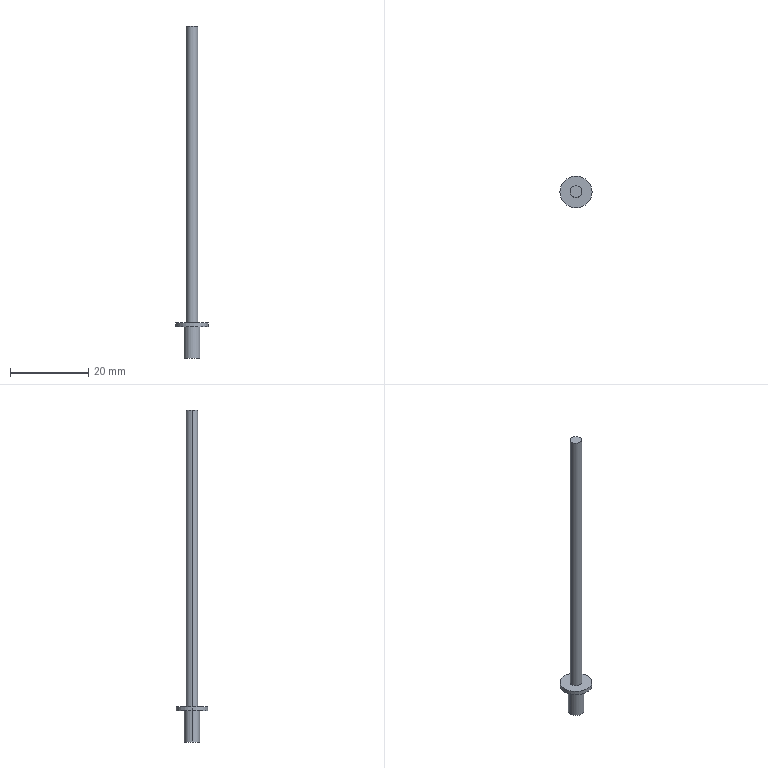Part | Creo | 1 solid | 10 faces | box 8.2 x 8.2 x 85 mm | volume 690.553 mm3 | cylinder 6 | plane 4 | commonest cylinder face diameters 3 x2 4 x2 8.2 x2
STEP:
#1=CARTESIAN_POINT('',(0.,0.,0.));
#2=DIRECTION('',(0.,0.,1.));
#3=DIRECTION('',(1.,0.,0.));
#4=AXIS2_PLACEMENT_3D('',#1,#2,#3);
#5=CARTESIAN_POINT('',(37.6,-82.,-54.09));
#6=VERTEX_POINT('',#5);
#7=CARTESIAN_POINT('',(29.4,-82.,-54.09));
#8=VERTEX_POINT('',#7);
#9=CARTESIAN_POINT('',(33.5,-82.,-54.09));
#10=DIRECTION('',(0.,0.,1.));
#11=DIRECTION('',(1.,0.,0.));
#12=AXIS2_PLACEMENT_3D('',#9,#10,#11);
#13=CIRCLE('',#12,4.1);
#14=EDGE_CURVE('',#6,#8,#13,.T.);
#15=ORIENTED_EDGE('',*,*,#14,.F.);
#16=CARTESIAN_POINT('',(33.5,-82.,-54.09));
#17=DIRECTION('',(0.,0.,1.));
#18=DIRECTION('',(-1.,0.,0.));
#19=AXIS2_PLACEMENT_3D('',#16,#17,#18);
#20=CIRCLE('',#19,4.1);
#21=EDGE_CURVE('',#8,#6,#20,.T.);
#22=ORIENTED_EDGE('',*,*,#21,.F.);
#23=EDGE_LOOP('',(#15,#22));
#24=FACE_OUTER_BOUND('',#23,.F.);
#25=CARTESIAN_POINT('',(35.,-82.,-54.09));
#26=VERTEX_POINT('',#25);
#27=CARTESIAN_POINT('',(32.,-82.,-54.09));
#28=VERTEX_POINT('',#27);
#29=CARTESIAN_POINT('',(33.5,-82.,-54.09));
#30=DIRECTION('',(0.,0.,-1.));
#31=DIRECTION('',(1.,0.,0.));
#32=AXIS2_PLACEMENT_3D('',#29,#30,#31);
#33=CIRCLE('',#32,1.5);
#34=EDGE_CURVE('',#26,#28,#33,.T.);
#35=ORIENTED_EDGE('',*,*,#34,.F.);
#36=CARTESIAN_POINT('',(33.5,-82.,-54.09));
#37=DIRECTION('',(0.,0.,-1.));
#38=DIRECTION('',(-1.,0.,0.));
#39=AXIS2_PLACEMENT_3D('',#36,#37,#38);
#40=CIRCLE('',#39,1.5);
#41=EDGE_CURVE('',#28,#26,#40,.T.);
#42=ORIENTED_EDGE('',*,*,#41,.F.);
#43=EDGE_LOOP('',(#35,#42));
#44=FACE_BOUND('',#43,.F.);
#45=CARTESIAN_POINT('',(33.5,-82.,-54.09));
#46=DIRECTION('',(0.,0.,1.));
#47=DIRECTION('',(1.,0.,0.));
#48=AXIS2_PLACEMENT_3D('',#45,#46,#47);
#49=PLANE('',#48);
#50=ADVANCED_FACE('',(#24,#44),#49,.T.);
#51=ORIENTED_EDGE('',*,*,#14,.T.);
#52=CARTESIAN_POINT('',(29.4,-82.,-55.09));
#53=VERTEX_POINT('',#52);
#54=CARTESIAN_POINT('',(29.4,-82.,-55.09));
#55=DIRECTION('',(0.,0.,1.));
#56=VECTOR('',#55,1.);
#57=LINE('',#54,#56);
#58=EDGE_CURVE('',#53,#8,#57,.T.);
#59=ORIENTED_EDGE('',*,*,#58,.F.);
#60=CARTESIAN_POINT('',(37.6,-82.,-55.09));
#61=VERTEX_POINT('',#60);
#62=CARTESIAN_POINT('',(33.5,-82.,-55.09));
#63=DIRECTION('',(0.,0.,-1.));
#64=DIRECTION('',(-1.,0.,0.));
#65=AXIS2_PLACEMENT_3D('',#62,#63,#64);
#66=CIRCLE('',#65,4.1);
#67=EDGE_CURVE('',#53,#61,#66,.T.);
#68=ORIENTED_EDGE('',*,*,#67,.T.);
#69=CARTESIAN_POINT('',(37.6,-82.,-55.09));
#70=DIRECTION('',(0.,0.,1.));
#71=VECTOR('',#70,1.);
#72=LINE('',#69,#71);
#73=EDGE_CURVE('',#61,#6,#72,.T.);
#74=ORIENTED_EDGE('',*,*,#73,.T.);
#75=EDGE_LOOP('',(#51,#59,#68,#74));
#76=FACE_OUTER_BOUND('',#75,.F.);
#77=CARTESIAN_POINT('',(33.5,-82.,-55.09));
#78=DIRECTION('',(0.,0.,1.));
#79=DIRECTION('',(1.,0.,0.));
#80=AXIS2_PLACEMENT_3D('',#77,#78,#79);
#81=CYLINDRICAL_SURFACE('',#80,4.1);
#82=ADVANCED_FACE('',(#76),#81,.T.);
#83=ORIENTED_EDGE('',*,*,#21,.T.);
#84=ORIENTED_EDGE('',*,*,#73,.F.);
#85=CARTESIAN_POINT('',(33.5,-82.,-55.09));
#86=DIRECTION('',(0.,0.,-1.));
#87=DIRECTION('',(1.,0.,0.));
#88=AXIS2_PLACEMENT_3D('',#85,#86,#87);
#89=CIRCLE('',#88,4.1);
#90=EDGE_CURVE('',#61,#53,#89,.T.);
#91=ORIENTED_EDGE('',*,*,#90,.T.);
#92=ORIENTED_EDGE('',*,*,#58,.T.);
#93=EDGE_LOOP('',(#83,#84,#91,#92));
#94=FACE_OUTER_BOUND('',#93,.F.);
#95=CARTESIAN_POINT('',(33.5,-82.,-55.09));
#96=DIRECTION('',(0.,0.,1.));
#97=DIRECTION('',(1.,0.,0.));
#98=AXIS2_PLACEMENT_3D('',#95,#96,#97);
#99=CYLINDRICAL_SURFACE('',#98,4.1);
#100=ADVANCED_FACE('',(#94),#99,.T.);
#101=ORIENTED_EDGE('',*,*,#90,.F.);
#102=ORIENTED_EDGE('',*,*,#67,.F.);
#103=EDGE_LOOP('',(#101,#102));
#104=FACE_OUTER_BOUND('',#103,.F.);
#105=CARTESIAN_POINT('',(35.5,-82.,-55.09));
#106=VERTEX_POINT('',#105);
#107=CARTESIAN_POINT('',(31.5,-82.,-55.09));
#108=VERTEX_POINT('',#107);
#109=CARTESIAN_POINT('',(33.5,-82.,-55.09));
#110=DIRECTION('',(0.,0.,1.));
#111=DIRECTION('',(1.,0.,0.));
#112=AXIS2_PLACEMENT_3D('',#109,#110,#111);
#113=CIRCLE('',#112,2.);
#114=EDGE_CURVE('',#106,#108,#113,.T.);
#115=ORIENTED_EDGE('',*,*,#114,.F.);
#116=CARTESIAN_POINT('',(33.5,-82.,-55.09));
#117=DIRECTION('',(0.,0.,1.));
#118=DIRECTION('',(-1.,0.,0.));
#119=AXIS2_PLACEMENT_3D('',#116,#117,#118);
#120=CIRCLE('',#119,2.);
#121=EDGE_CURVE('',#108,#106,#120,.T.);
#122=ORIENTED_EDGE('',*,*,#121,.F.);
#123=EDGE_LOOP('',(#115,#122));
#124=FACE_BOUND('',#123,.F.);
#125=CARTESIAN_POINT('',(33.5,-82.,-55.09));
#126=DIRECTION('',(0.,0.,-1.));
#127=DIRECTION('',(-1.,0.,0.));
#128=AXIS2_PLACEMENT_3D('',#125,#126,#127);
#129=PLANE('',#128);
#130=ADVANCED_FACE('',(#104,#124),#129,.T.);
#131=CARTESIAN_POINT('',(31.5,-82.,-63.09));
#132=VERTEX_POINT('',#131);
#133=CARTESIAN_POINT('',(35.5,-82.,-63.09));
#134=VERTEX_POINT('',#133);
#135=CARTESIAN_POINT('',(33.5,-82.,-63.09));
#136=DIRECTION('',(0.,0.,-1.));
#137=DIRECTION('',(-1.,0.,0.));
#138=AXIS2_PLACEMENT_3D('',#135,#136,#137);
#139=CIRCLE('',#138,2.);
#140=EDGE_CURVE('',#132,#134,#139,.T.);
#141=ORIENTED_EDGE('',*,*,#140,.T.);
#142=CARTESIAN_POINT('',(35.5,-82.,-63.09));
#143=DIRECTION('',(0.,0.,1.));
#144=VECTOR('',#143,8.);
#145=LINE('',#142,#144);
#146=EDGE_CURVE('',#134,#106,#145,.T.);
#147=ORIENTED_EDGE('',*,*,#146,.T.);
#148=ORIENTED_EDGE('',*,*,#114,.T.);
#149=CARTESIAN_POINT('',(31.5,-82.,-63.09));
#150=DIRECTION('',(0.,0.,1.));
#151=VECTOR('',#150,8.);
#152=LINE('',#149,#151);
#153=EDGE_CURVE('',#132,#108,#152,.T.);
#154=ORIENTED_EDGE('',*,*,#153,.F.);
#155=EDGE_LOOP('',(#141,#147,#148,#154));
#156=FACE_OUTER_BOUND('',#155,.F.);
#157=CARTESIAN_POINT('',(33.5,-82.,-90.09));
#158=DIRECTION('',(0.,0.,1.));
#159=DIRECTION('',(1.,0.,0.));
#160=AXIS2_PLACEMENT_3D('',#157,#158,#159);
#161=CYLINDRICAL_SURFACE('',#160,2.);
#162=ADVANCED_FACE('',(#156),#161,.T.);
#163=CARTESIAN_POINT('',(33.5,-82.,-63.09));
#164=DIRECTION('',(0.,0.,-1.));
#165=DIRECTION('',(1.,0.,0.));
#166=AXIS2_PLACEMENT_3D('',#163,#164,#165);
#167=CIRCLE('',#166,2.);
#168=EDGE_CURVE('',#134,#132,#167,.T.);
#169=ORIENTED_EDGE('',*,*,#168,.F.);
#170=ORIENTED_EDGE('',*,*,#140,.F.);
#171=EDGE_LOOP('',(#169,#170));
#172=FACE_OUTER_BOUND('',#171,.F.);
#173=CARTESIAN_POINT('',(-38.5,-81.,-63.09));
#174=DIRECTION('',(0.,0.,1.));
#175=DIRECTION('',(1.,0.,0.));
#176=AXIS2_PLACEMENT_3D('',#173,#174,#175);
#177=PLANE('',#176);
#178=ADVANCED_FACE('',(#172),#177,.F.);
#179=ORIENTED_EDGE('',*,*,#168,.T.);
#180=ORIENTED_EDGE('',*,*,#153,.T.);
#181=ORIENTED_EDGE('',*,*,#121,.T.);
#182=ORIENTED_EDGE('',*,*,#146,.F.);
#183=EDGE_LOOP('',(#179,#180,#181,#182));
#184=FACE_OUTER_BOUND('',#183,.F.);
#185=CARTESIAN_POINT('',(33.5,-82.,-90.09));
#186=DIRECTION('',(0.,0.,1.));
#187=DIRECTION('',(1.,0.,0.));
#188=AXIS2_PLACEMENT_3D('',#185,#186,#187);
#189=CYLINDRICAL_SURFACE('',#188,2.);
#190=ADVANCED_FACE('',(#184),#189,.T.);
#191=ORIENTED_EDGE('',*,*,#34,.T.);
#192=CARTESIAN_POINT('',(32.,-82.,21.91));
#193=VERTEX_POINT('',#192);
#194=CARTESIAN_POINT('',(32.,-82.,21.91));
#195=DIRECTION('',(0.,0.,-1.));
#196=VECTOR('',#195,76.);
#197=LINE('',#194,#196);
#198=EDGE_CURVE('',#193,#28,#197,.T.);
#199=ORIENTED_EDGE('',*,*,#198,.F.);
#200=CARTESIAN_POINT('',(35.,-82.,21.91));
#201=VERTEX_POINT('',#200);
#202=CARTESIAN_POINT('',(33.5,-82.,21.91));
#203=DIRECTION('',(0.,0.,1.));
#204=DIRECTION('',(-1.,0.,0.));
#205=AXIS2_PLACEMENT_3D('',#202,#203,#204);
#206=CIRCLE('',#205,1.5);
#207=EDGE_CURVE('',#193,#201,#206,.T.);
#208=ORIENTED_EDGE('',*,*,#207,.T.);
#209=CARTESIAN_POINT('',(35.,-82.,21.91));
#210=DIRECTION('',(0.,0.,-1.));
#211=VECTOR('',#210,76.);
#212=LINE('',#209,#211);
#213=EDGE_CURVE('',#201,#26,#212,.T.);
#214=ORIENTED_EDGE('',*,*,#213,.T.);
#215=EDGE_LOOP('',(#191,#199,#208,#214));
#216=FACE_OUTER_BOUND('',#215,.F.);
#217=CARTESIAN_POINT('',(33.5,-82.,11.91));
#218=DIRECTION('',(0.,0.,-1.));
#219=DIRECTION('',(-1.,0.,0.));
#220=AXIS2_PLACEMENT_3D('',#217,#218,#219);
#221=CYLINDRICAL_SURFACE('',#220,1.5);
#222=ADVANCED_FACE('',(#216),#221,.T.);
#223=ORIENTED_EDGE('',*,*,#41,.T.);
#224=ORIENTED_EDGE('',*,*,#213,.F.);
#225=CARTESIAN_POINT('',(33.5,-82.,21.91));
#226=DIRECTION('',(0.,0.,1.));
#227=DIRECTION('',(1.,0.,0.));
#228=AXIS2_PLACEMENT_3D('',#225,#226,#227);
#229=CIRCLE('',#228,1.5);
#230=EDGE_CURVE('',#201,#193,#229,.T.);
#231=ORIENTED_EDGE('',*,*,#230,.T.);
#232=ORIENTED_EDGE('',*,*,#198,.T.);
#233=EDGE_LOOP('',(#223,#224,#231,#232));
#234=FACE_OUTER_BOUND('',#233,.F.);
#235=CARTESIAN_POINT('',(33.5,-82.,11.91));
#236=DIRECTION('',(0.,0.,-1.));
#237=DIRECTION('',(-1.,0.,0.));
#238=AXIS2_PLACEMENT_3D('',#235,#236,#237);
#239=CYLINDRICAL_SURFACE('',#238,1.5);
#240=ADVANCED_FACE('',(#234),#239,.T.);
#241=ORIENTED_EDGE('',*,*,#230,.F.);
#242=ORIENTED_EDGE('',*,*,#207,.F.);
#243=EDGE_LOOP('',(#241,#242));
#244=FACE_OUTER_BOUND('',#243,.F.);
#245=CARTESIAN_POINT('',(33.5,-82.,21.91));
#246=DIRECTION('',(0.,0.,1.));
#247=DIRECTION('',(1.,0.,0.));
#248=AXIS2_PLACEMENT_3D('',#245,#246,#247);
#249=PLANE('',#248);
#250=ADVANCED_FACE('',(#244),#249,.T.);
#251=CLOSED_SHELL('',(#50,#82,#100,#130,#162,#178,#190,#222,#240,#250));
#252=MANIFOLD_SOLID_BREP('',#251);
#253=(LENGTH_UNIT()NAMED_UNIT(*)SI_UNIT(.MILLI.,.METRE.));
#254=UNCERTAINTY_MEASURE_WITH_UNIT(LENGTH_MEASURE(0.008578),#253,'','');
#255=(NAMED_UNIT(*)PLANE_ANGLE_UNIT()SI_UNIT($,.RADIAN.));
#256=PLANE_ANGLE_MEASURE_WITH_UNIT(PLANE_ANGLE_MEASURE(0.01745),#255);
#257=(CONVERSION_BASED_UNIT('DEGREE',#256)NAMED_UNIT(*)PLANE_ANGLE_UNIT());
#258=(NAMED_UNIT(*)SI_UNIT($,.STERADIAN.)SOLID_ANGLE_UNIT());
#259=(GEOMETRIC_REPRESENTATION_CONTEXT(3)GLOBAL_UNCERTAINTY_ASSIGNED_CONTEXT((#254))GLOBAL_UNIT_ASSIGNED_CONTEXT((#253,#257,#258))REPRESENTATION_CONTEXT('',''));
#260=ADVANCED_BREP_SHAPE_REPRESENTATION('',(#4,#252),#259);